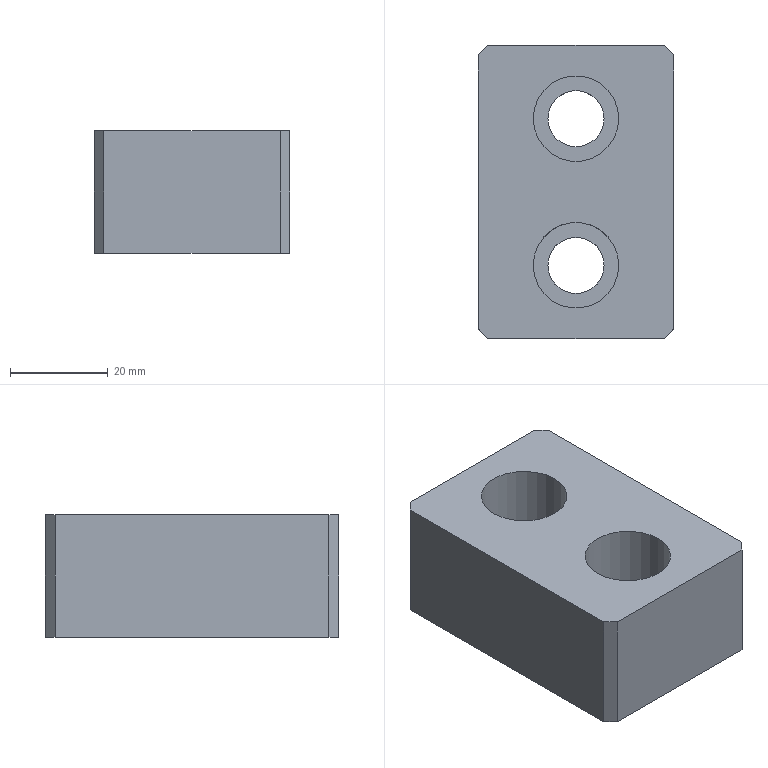Part | NX | features solid 2 | 1 solid | 16 faces | box 40 x 60 x 25 mm | volume 50507 mm3 | plane 12 | cylinder 4 | commonest cylinder face diameters 11.5 x2 17.5 x2
STEP:
#1=CARTESIAN_POINT('',(785.,-162.,435.));
#2=VERTEX_POINT('',#1);
#3=CARTESIAN_POINT('',(785.,-218.,435.));
#4=VERTEX_POINT('',#3);
#5=CARTESIAN_POINT('',(785.,-160.,435.));
#6=DIRECTION('',(0.,-1.,0.));
#7=VECTOR('',#6,1000.);
#8=LINE('',#5,#7);
#9=EDGE_CURVE('',#2,#4,#8,.T.);
#10=ORIENTED_EDGE('',*,*,#9,.F.);
#11=CARTESIAN_POINT('',(785.,-162.,460.));
#12=VERTEX_POINT('',#11);
#13=CARTESIAN_POINT('',(785.,-162.,435.));
#14=DIRECTION('',(0.,0.,1.));
#15=VECTOR('',#14,1000.);
#16=LINE('',#13,#15);
#17=EDGE_CURVE('',#2,#12,#16,.T.);
#18=ORIENTED_EDGE('',*,*,#17,.T.);
#19=CARTESIAN_POINT('',(785.,-218.,460.));
#20=VERTEX_POINT('',#19);
#21=CARTESIAN_POINT('',(785.,0.,460.));
#22=DIRECTION('',(0.,-1.,0.));
#23=VECTOR('',#22,1000.);
#24=LINE('',#21,#23);
#25=EDGE_CURVE('',#12,#20,#24,.T.);
#26=ORIENTED_EDGE('',*,*,#25,.T.);
#27=CARTESIAN_POINT('',(785.,-218.,435.));
#28=DIRECTION('',(0.,0.,-1.));
#29=VECTOR('',#28,1000.);
#30=LINE('',#27,#29);
#31=EDGE_CURVE('',#20,#4,#30,.T.);
#32=ORIENTED_EDGE('',*,*,#31,.T.);
#33=EDGE_LOOP('',(#10,#18,#26,#32));
#34=FACE_BOUND('',#33,.T.);
#35=CARTESIAN_POINT('',(785.,-160.,435.));
#36=DIRECTION('',(-1.,0.,0.));
#37=DIRECTION('',(0.,0.,1.));
#38=AXIS2_PLACEMENT_3D('',#35,#36,#37);
#39=PLANE('',#38);
#40=ADVANCED_FACE('',(#34),#39,.F.);
#41=CARTESIAN_POINT('',(747.,-160.,435.));
#42=VERTEX_POINT('',#41);
#43=CARTESIAN_POINT('',(783.,-160.,435.));
#44=VERTEX_POINT('',#43);
#45=CARTESIAN_POINT('',(745.,-160.,435.));
#46=DIRECTION('',(1.,0.,0.));
#47=VECTOR('',#46,1000.);
#48=LINE('',#45,#47);
#49=EDGE_CURVE('',#42,#44,#48,.T.);
#50=ORIENTED_EDGE('',*,*,#49,.F.);
#51=CARTESIAN_POINT('',(747.,-160.,460.));
#52=VERTEX_POINT('',#51);
#53=CARTESIAN_POINT('',(747.,-160.,435.));
#54=DIRECTION('',(0.,0.,1.));
#55=VECTOR('',#54,1000.);
#56=LINE('',#53,#55);
#57=EDGE_CURVE('',#42,#52,#56,.T.);
#58=ORIENTED_EDGE('',*,*,#57,.T.);
#59=CARTESIAN_POINT('',(783.,-160.,460.));
#60=VERTEX_POINT('',#59);
#61=CARTESIAN_POINT('',(0.,-160.,460.));
#62=DIRECTION('',(1.,0.,0.));
#63=VECTOR('',#62,1000.);
#64=LINE('',#61,#63);
#65=EDGE_CURVE('',#52,#60,#64,.T.);
#66=ORIENTED_EDGE('',*,*,#65,.T.);
#67=CARTESIAN_POINT('',(783.,-160.,435.));
#68=DIRECTION('',(0.,0.,-1.));
#69=VECTOR('',#68,1000.);
#70=LINE('',#67,#69);
#71=EDGE_CURVE('',#60,#44,#70,.T.);
#72=ORIENTED_EDGE('',*,*,#71,.T.);
#73=EDGE_LOOP('',(#50,#58,#66,#72));
#74=FACE_BOUND('',#73,.T.);
#75=CARTESIAN_POINT('',(745.,-160.,435.));
#76=DIRECTION('',(0.,-1.,0.));
#77=DIRECTION('',(0.,0.,-1.));
#78=AXIS2_PLACEMENT_3D('',#75,#76,#77);
#79=PLANE('',#78);
#80=ADVANCED_FACE('',(#74),#79,.F.);
#81=CARTESIAN_POINT('',(745.,-218.,460.));
#82=VERTEX_POINT('',#81);
#83=CARTESIAN_POINT('',(745.,-162.,460.));
#84=VERTEX_POINT('',#83);
#85=CARTESIAN_POINT('',(745.,0.,460.));
#86=DIRECTION('',(0.,-1.,0.));
#87=VECTOR('',#86,1000.);
#88=LINE('',#85,#87);
#89=EDGE_CURVE('',#82,#84,#88,.F.);
#90=ORIENTED_EDGE('',*,*,#89,.T.);
#91=CARTESIAN_POINT('',(745.,-162.,435.));
#92=VERTEX_POINT('',#91);
#93=CARTESIAN_POINT('',(745.,-162.,435.));
#94=DIRECTION('',(0.,0.,1.));
#95=VECTOR('',#94,1000.);
#96=LINE('',#93,#95);
#97=EDGE_CURVE('',#84,#92,#96,.F.);
#98=ORIENTED_EDGE('',*,*,#97,.T.);
#99=CARTESIAN_POINT('',(745.,-218.,435.));
#100=VERTEX_POINT('',#99);
#101=CARTESIAN_POINT('',(745.,-160.,435.));
#102=DIRECTION('',(0.,-1.,0.));
#103=VECTOR('',#102,1000.);
#104=LINE('',#101,#103);
#105=EDGE_CURVE('',#100,#92,#104,.F.);
#106=ORIENTED_EDGE('',*,*,#105,.F.);
#107=CARTESIAN_POINT('',(745.,-218.,460.));
#108=DIRECTION('',(0.,0.,-1.));
#109=VECTOR('',#108,1000.);
#110=LINE('',#107,#109);
#111=EDGE_CURVE('',#100,#82,#110,.F.);
#112=ORIENTED_EDGE('',*,*,#111,.T.);
#113=EDGE_LOOP('',(#90,#98,#106,#112));
#114=FACE_BOUND('',#113,.T.);
#115=CARTESIAN_POINT('',(745.,-160.,435.));
#116=DIRECTION('',(-1.,0.,0.));
#117=DIRECTION('',(0.,0.,1.));
#118=AXIS2_PLACEMENT_3D('',#115,#116,#117);
#119=PLANE('',#118);
#120=ADVANCED_FACE('',(#114),#119,.T.);
#121=CARTESIAN_POINT('',(747.,-220.,435.));
#122=VERTEX_POINT('',#121);
#123=CARTESIAN_POINT('',(783.,-220.,435.));
#124=VERTEX_POINT('',#123);
#125=CARTESIAN_POINT('',(745.,-220.,435.));
#126=DIRECTION('',(1.,0.,0.));
#127=VECTOR('',#126,1000.);
#128=LINE('',#125,#127);
#129=EDGE_CURVE('',#122,#124,#128,.T.);
#130=ORIENTED_EDGE('',*,*,#129,.T.);
#131=CARTESIAN_POINT('',(783.,-220.,460.));
#132=VERTEX_POINT('',#131);
#133=CARTESIAN_POINT('',(783.,-220.,460.));
#134=DIRECTION('',(0.,0.,1.));
#135=VECTOR('',#134,1000.);
#136=LINE('',#133,#135);
#137=EDGE_CURVE('',#124,#132,#136,.T.);
#138=ORIENTED_EDGE('',*,*,#137,.T.);
#139=CARTESIAN_POINT('',(747.,-220.,460.));
#140=VERTEX_POINT('',#139);
#141=CARTESIAN_POINT('',(0.,-220.,460.));
#142=DIRECTION('',(1.,0.,0.));
#143=VECTOR('',#142,1000.);
#144=LINE('',#141,#143);
#145=EDGE_CURVE('',#140,#132,#144,.T.);
#146=ORIENTED_EDGE('',*,*,#145,.F.);
#147=CARTESIAN_POINT('',(747.,-220.,435.));
#148=DIRECTION('',(0.,0.,-1.));
#149=VECTOR('',#148,1000.);
#150=LINE('',#147,#149);
#151=EDGE_CURVE('',#140,#122,#150,.T.);
#152=ORIENTED_EDGE('',*,*,#151,.T.);
#153=EDGE_LOOP('',(#130,#138,#146,#152));
#154=FACE_BOUND('',#153,.T.);
#155=CARTESIAN_POINT('',(745.,-220.,435.));
#156=DIRECTION('',(0.,-1.,0.));
#157=DIRECTION('',(0.,0.,-1.));
#158=AXIS2_PLACEMENT_3D('',#155,#156,#157);
#159=PLANE('',#158);
#160=ADVANCED_FACE('',(#154),#159,.T.);
#161=CARTESIAN_POINT('',(770.75,-205.,435.));
#162=VERTEX_POINT('',#161);
#163=CARTESIAN_POINT('',(765.,-205.,435.));
#164=DIRECTION('',(0.,0.,1.));
#165=DIRECTION('',(1.,0.,0.));
#166=AXIS2_PLACEMENT_3D('',#163,#164,#165);
#167=CIRCLE('',#166,5.75);
#168=EDGE_CURVE('',#162,#162,#167,.T.);
#169=ORIENTED_EDGE('',*,*,#168,.T.);
#170=EDGE_LOOP('',(#169));
#171=FACE_BOUND('',#170,.T.);
#172=CARTESIAN_POINT('',(770.75,-175.,435.));
#173=VERTEX_POINT('',#172);
#174=CARTESIAN_POINT('',(765.,-175.,435.));
#175=DIRECTION('',(0.,0.,1.));
#176=DIRECTION('',(1.,0.,0.));
#177=AXIS2_PLACEMENT_3D('',#174,#175,#176);
#178=CIRCLE('',#177,5.75);
#179=EDGE_CURVE('',#173,#173,#178,.T.);
#180=ORIENTED_EDGE('',*,*,#179,.T.);
#181=EDGE_LOOP('',(#180));
#182=FACE_BOUND('',#181,.T.);
#183=ORIENTED_EDGE('',*,*,#105,.T.);
#184=CARTESIAN_POINT('',(747.,-160.,435.));
#185=DIRECTION('',(0.7071,0.7071,0.));
#186=VECTOR('',#185,1000.);
#187=LINE('',#184,#186);
#188=EDGE_CURVE('',#92,#42,#187,.T.);
#189=ORIENTED_EDGE('',*,*,#188,.T.);
#190=ORIENTED_EDGE('',*,*,#49,.T.);
#191=CARTESIAN_POINT('',(785.,-162.,435.));
#192=DIRECTION('',(-0.7071,0.7071,0.));
#193=VECTOR('',#192,1000.);
#194=LINE('',#191,#193);
#195=EDGE_CURVE('',#44,#2,#194,.F.);
#196=ORIENTED_EDGE('',*,*,#195,.T.);
#197=ORIENTED_EDGE('',*,*,#9,.T.);
#198=CARTESIAN_POINT('',(783.,-220.,435.));
#199=DIRECTION('',(-0.7071,-0.7071,0.));
#200=VECTOR('',#199,1000.);
#201=LINE('',#198,#200);
#202=EDGE_CURVE('',#4,#124,#201,.T.);
#203=ORIENTED_EDGE('',*,*,#202,.T.);
#204=ORIENTED_EDGE('',*,*,#129,.F.);
#205=CARTESIAN_POINT('',(745.,-218.,435.));
#206=DIRECTION('',(0.7071,-0.7071,0.));
#207=VECTOR('',#206,1000.);
#208=LINE('',#205,#207);
#209=EDGE_CURVE('',#122,#100,#208,.F.);
#210=ORIENTED_EDGE('',*,*,#209,.T.);
#211=EDGE_LOOP('',(#183,#189,#190,#196,#197,#203,#204,#210));
#212=FACE_BOUND('',#211,.T.);
#213=CARTESIAN_POINT('',(745.,-160.,435.));
#214=DIRECTION('',(0.,0.,1.));
#215=DIRECTION('',(0.,-1.,0.));
#216=AXIS2_PLACEMENT_3D('',#213,#214,#215);
#217=PLANE('',#216);
#218=ADVANCED_FACE('',(#171,#182,#212),#217,.F.);
#219=CARTESIAN_POINT('',(756.25,-205.,460.));
#220=VERTEX_POINT('',#219);
#221=CARTESIAN_POINT('',(765.,-205.,460.));
#222=DIRECTION('',(0.,0.,-1.));
#223=DIRECTION('',(-1.,0.,0.));
#224=AXIS2_PLACEMENT_3D('',#221,#222,#223);
#225=CIRCLE('',#224,8.75);
#226=EDGE_CURVE('',#220,#220,#225,.T.);
#227=ORIENTED_EDGE('',*,*,#226,.T.);
#228=EDGE_LOOP('',(#227));
#229=FACE_BOUND('',#228,.T.);
#230=CARTESIAN_POINT('',(756.25,-175.,460.));
#231=VERTEX_POINT('',#230);
#232=CARTESIAN_POINT('',(765.,-175.,460.));
#233=DIRECTION('',(0.,0.,-1.));
#234=DIRECTION('',(-1.,0.,0.));
#235=AXIS2_PLACEMENT_3D('',#232,#233,#234);
#236=CIRCLE('',#235,8.75);
#237=EDGE_CURVE('',#231,#231,#236,.T.);
#238=ORIENTED_EDGE('',*,*,#237,.T.);
#239=EDGE_LOOP('',(#238));
#240=FACE_BOUND('',#239,.T.);
#241=ORIENTED_EDGE('',*,*,#65,.F.);
#242=CARTESIAN_POINT('',(453.5,-453.5,460.));
#243=DIRECTION('',(-0.7071,-0.7071,0.));
#244=VECTOR('',#243,1000.);
#245=LINE('',#242,#244);
#246=EDGE_CURVE('',#52,#84,#245,.T.);
#247=ORIENTED_EDGE('',*,*,#246,.T.);
#248=ORIENTED_EDGE('',*,*,#89,.F.);
#249=CARTESIAN_POINT('',(263.5,263.5,460.));
#250=DIRECTION('',(-0.7071,0.7071,0.));
#251=VECTOR('',#250,1000.);
#252=LINE('',#249,#251);
#253=EDGE_CURVE('',#82,#140,#252,.F.);
#254=ORIENTED_EDGE('',*,*,#253,.T.);
#255=ORIENTED_EDGE('',*,*,#145,.T.);
#256=CARTESIAN_POINT('',(501.5,-501.5,460.));
#257=DIRECTION('',(0.7071,0.7071,0.));
#258=VECTOR('',#257,1000.);
#259=LINE('',#256,#258);
#260=EDGE_CURVE('',#132,#20,#259,.T.);
#261=ORIENTED_EDGE('',*,*,#260,.T.);
#262=ORIENTED_EDGE('',*,*,#25,.F.);
#263=CARTESIAN_POINT('',(311.5,311.5,460.));
#264=DIRECTION('',(0.7071,-0.7071,0.));
#265=VECTOR('',#264,1000.);
#266=LINE('',#263,#265);
#267=EDGE_CURVE('',#12,#60,#266,.F.);
#268=ORIENTED_EDGE('',*,*,#267,.T.);
#269=EDGE_LOOP('',(#241,#247,#248,#254,#255,#261,#262,#268));
#270=FACE_BOUND('',#269,.T.);
#271=CARTESIAN_POINT('',(0.,0.,460.));
#272=DIRECTION('',(0.,0.,1.));
#273=DIRECTION('',(1.,0.,0.));
#274=AXIS2_PLACEMENT_3D('',#271,#272,#273);
#275=PLANE('',#274);
#276=ADVANCED_FACE('',(#229,#240,#270),#275,.T.);
#277=ORIENTED_EDGE('',*,*,#188,.F.);
#278=ORIENTED_EDGE('',*,*,#97,.F.);
#279=ORIENTED_EDGE('',*,*,#246,.F.);
#280=ORIENTED_EDGE('',*,*,#57,.F.);
#281=EDGE_LOOP('',(#277,#278,#279,#280));
#282=FACE_BOUND('',#281,.T.);
#283=CARTESIAN_POINT('',(747.,-160.,435.));
#284=DIRECTION('',(-0.7071,0.7071,0.));
#285=DIRECTION('',(-0.7071,-0.7071,0.));
#286=AXIS2_PLACEMENT_3D('',#283,#284,#285);
#287=PLANE('',#286);
#288=ADVANCED_FACE('',(#282),#287,.T.);
#289=ORIENTED_EDGE('',*,*,#195,.F.);
#290=ORIENTED_EDGE('',*,*,#71,.F.);
#291=ORIENTED_EDGE('',*,*,#267,.F.);
#292=ORIENTED_EDGE('',*,*,#17,.F.);
#293=EDGE_LOOP('',(#289,#290,#291,#292));
#294=FACE_BOUND('',#293,.T.);
#295=CARTESIAN_POINT('',(785.,-162.,435.));
#296=DIRECTION('',(-0.7071,-0.7071,0.));
#297=DIRECTION('',(0.7071,-0.7071,0.));
#298=AXIS2_PLACEMENT_3D('',#295,#296,#297);
#299=PLANE('',#298);
#300=ADVANCED_FACE('',(#294),#299,.F.);
#301=ORIENTED_EDGE('',*,*,#202,.F.);
#302=ORIENTED_EDGE('',*,*,#31,.F.);
#303=ORIENTED_EDGE('',*,*,#260,.F.);
#304=ORIENTED_EDGE('',*,*,#137,.F.);
#305=EDGE_LOOP('',(#301,#302,#303,#304));
#306=FACE_BOUND('',#305,.T.);
#307=CARTESIAN_POINT('',(783.,-220.,435.));
#308=DIRECTION('',(0.7071,-0.7071,0.));
#309=DIRECTION('',(0.7071,0.7071,0.));
#310=AXIS2_PLACEMENT_3D('',#307,#308,#309);
#311=PLANE('',#310);
#312=ADVANCED_FACE('',(#306),#311,.T.);
#313=ORIENTED_EDGE('',*,*,#209,.F.);
#314=ORIENTED_EDGE('',*,*,#151,.F.);
#315=ORIENTED_EDGE('',*,*,#253,.F.);
#316=ORIENTED_EDGE('',*,*,#111,.F.);
#317=EDGE_LOOP('',(#313,#314,#315,#316));
#318=FACE_BOUND('',#317,.T.);
#319=CARTESIAN_POINT('',(745.,-218.,435.));
#320=DIRECTION('',(0.7071,0.7071,0.));
#321=DIRECTION('',(-0.7071,0.7071,0.));
#322=AXIS2_PLACEMENT_3D('',#319,#320,#321);
#323=PLANE('',#322);
#324=ADVANCED_FACE('',(#318),#323,.F.);
#325=CARTESIAN_POINT('',(759.25,-175.,445.));
#326=VERTEX_POINT('',#325);
#327=CARTESIAN_POINT('',(765.,-175.,445.));
#328=DIRECTION('',(0.,0.,-1.));
#329=DIRECTION('',(-1.,0.,0.));
#330=AXIS2_PLACEMENT_3D('',#327,#328,#329);
#331=CIRCLE('',#330,5.75);
#332=EDGE_CURVE('',#326,#326,#331,.T.);
#333=ORIENTED_EDGE('',*,*,#332,.F.);
#334=EDGE_LOOP('',(#333));
#335=FACE_BOUND('',#334,.T.);
#336=ORIENTED_EDGE('',*,*,#179,.F.);
#337=EDGE_LOOP('',(#336));
#338=FACE_BOUND('',#337,.T.);
#339=CARTESIAN_POINT('',(765.,-175.,260.));
#340=DIRECTION('',(0.,0.,-1.));
#341=DIRECTION('',(-1.,0.,0.));
#342=AXIS2_PLACEMENT_3D('',#339,#340,#341);
#343=CYLINDRICAL_SURFACE('',#342,5.75);
#344=ADVANCED_FACE('',(#335,#338),#343,.F.);
#345=ORIENTED_EDGE('',*,*,#332,.T.);
#346=EDGE_LOOP('',(#345));
#347=FACE_BOUND('',#346,.T.);
#348=CARTESIAN_POINT('',(756.25,-175.,445.));
#349=VERTEX_POINT('',#348);
#350=CARTESIAN_POINT('',(765.,-175.,445.));
#351=DIRECTION('',(0.,0.,-1.));
#352=DIRECTION('',(-1.,0.,0.));
#353=AXIS2_PLACEMENT_3D('',#350,#351,#352);
#354=CIRCLE('',#353,8.75);
#355=EDGE_CURVE('',#349,#349,#354,.T.);
#356=ORIENTED_EDGE('',*,*,#355,.F.);
#357=EDGE_LOOP('',(#356));
#358=FACE_BOUND('',#357,.T.);
#359=CARTESIAN_POINT('',(765.,-175.,445.));
#360=DIRECTION('',(0.,0.,-1.));
#361=DIRECTION('',(-1.,0.,0.));
#362=AXIS2_PLACEMENT_3D('',#359,#360,#361);
#363=PLANE('',#362);
#364=ADVANCED_FACE('',(#347,#358),#363,.F.);
#365=ORIENTED_EDGE('',*,*,#355,.T.);
#366=EDGE_LOOP('',(#365));
#367=FACE_BOUND('',#366,.T.);
#368=ORIENTED_EDGE('',*,*,#237,.F.);
#369=EDGE_LOOP('',(#368));
#370=FACE_BOUND('',#369,.T.);
#371=CARTESIAN_POINT('',(765.,-175.,460.));
#372=DIRECTION('',(0.,0.,-1.));
#373=DIRECTION('',(-1.,0.,0.));
#374=AXIS2_PLACEMENT_3D('',#371,#372,#373);
#375=CYLINDRICAL_SURFACE('',#374,8.75);
#376=ADVANCED_FACE('',(#367,#370),#375,.F.);
#377=CARTESIAN_POINT('',(759.25,-205.,445.));
#378=VERTEX_POINT('',#377);
#379=CARTESIAN_POINT('',(765.,-205.,445.));
#380=DIRECTION('',(0.,0.,-1.));
#381=DIRECTION('',(-1.,0.,0.));
#382=AXIS2_PLACEMENT_3D('',#379,#380,#381);
#383=CIRCLE('',#382,5.75);
#384=EDGE_CURVE('',#378,#378,#383,.T.);
#385=ORIENTED_EDGE('',*,*,#384,.F.);
#386=EDGE_LOOP('',(#385));
#387=FACE_BOUND('',#386,.T.);
#388=ORIENTED_EDGE('',*,*,#168,.F.);
#389=EDGE_LOOP('',(#388));
#390=FACE_BOUND('',#389,.T.);
#391=CARTESIAN_POINT('',(765.,-205.,260.));
#392=DIRECTION('',(0.,0.,-1.));
#393=DIRECTION('',(-1.,0.,0.));
#394=AXIS2_PLACEMENT_3D('',#391,#392,#393);
#395=CYLINDRICAL_SURFACE('',#394,5.75);
#396=ADVANCED_FACE('',(#387,#390),#395,.F.);
#397=ORIENTED_EDGE('',*,*,#384,.T.);
#398=EDGE_LOOP('',(#397));
#399=FACE_BOUND('',#398,.T.);
#400=CARTESIAN_POINT('',(756.25,-205.,445.));
#401=VERTEX_POINT('',#400);
#402=CARTESIAN_POINT('',(765.,-205.,445.));
#403=DIRECTION('',(0.,0.,-1.));
#404=DIRECTION('',(-1.,0.,0.));
#405=AXIS2_PLACEMENT_3D('',#402,#403,#404);
#406=CIRCLE('',#405,8.75);
#407=EDGE_CURVE('',#401,#401,#406,.T.);
#408=ORIENTED_EDGE('',*,*,#407,.F.);
#409=EDGE_LOOP('',(#408));
#410=FACE_BOUND('',#409,.T.);
#411=CARTESIAN_POINT('',(765.,-205.,445.));
#412=DIRECTION('',(0.,0.,-1.));
#413=DIRECTION('',(-1.,0.,0.));
#414=AXIS2_PLACEMENT_3D('',#411,#412,#413);
#415=PLANE('',#414);
#416=ADVANCED_FACE('',(#399,#410),#415,.F.);
#417=ORIENTED_EDGE('',*,*,#407,.T.);
#418=EDGE_LOOP('',(#417));
#419=FACE_BOUND('',#418,.T.);
#420=ORIENTED_EDGE('',*,*,#226,.F.);
#421=EDGE_LOOP('',(#420));
#422=FACE_BOUND('',#421,.T.);
#423=CARTESIAN_POINT('',(765.,-205.,460.));
#424=DIRECTION('',(0.,0.,-1.));
#425=DIRECTION('',(-1.,0.,0.));
#426=AXIS2_PLACEMENT_3D('',#423,#424,#425);
#427=CYLINDRICAL_SURFACE('',#426,8.75);
#428=ADVANCED_FACE('',(#419,#422),#427,.F.);
#429=CLOSED_SHELL('',(#40,#80,#120,#160,#218,#276,#288,#300,#312,#324,#344,#364,#376,#396,#416,#428));
#430=MANIFOLD_SOLID_BREP('',#429);
#431=(LENGTH_UNIT()NAMED_UNIT(*)SI_UNIT(.MILLI.,.METRE.));
#432=UNCERTAINTY_MEASURE_WITH_UNIT(LENGTH_MEASURE(0.00001),#431,'','');
#433=(NAMED_UNIT(*)PLANE_ANGLE_UNIT()SI_UNIT($,.RADIAN.));
#434=(NAMED_UNIT(*)SI_UNIT($,.STERADIAN.)SOLID_ANGLE_UNIT());
#435=(GEOMETRIC_REPRESENTATION_CONTEXT(3)GLOBAL_UNCERTAINTY_ASSIGNED_CONTEXT((#432))GLOBAL_UNIT_ASSIGNED_CONTEXT((#431,#433,#434))REPRESENTATION_CONTEXT('',''));
#436=ADVANCED_BREP_SHAPE_REPRESENTATION('',(#430),#435);